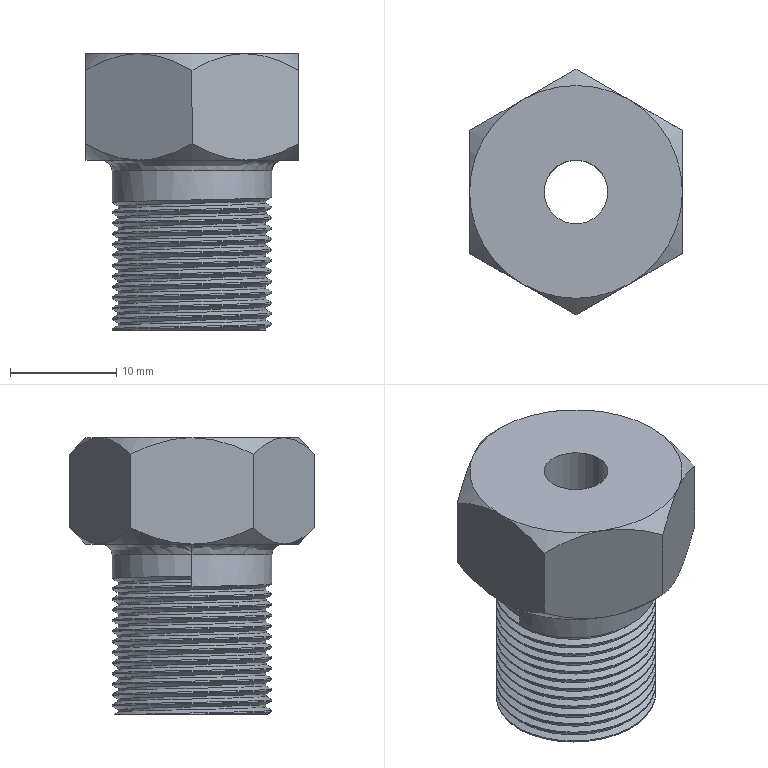Part | SolidWorks | features BaseBody 1 | 1 solid | 59 faces | box 20 x 23.094 x 26 mm | volume 5258 mm3 | cylinder 29 | cone 14 | plane 11 | spline 5 | commonest cylinder face diameters 15 x27 6 x2